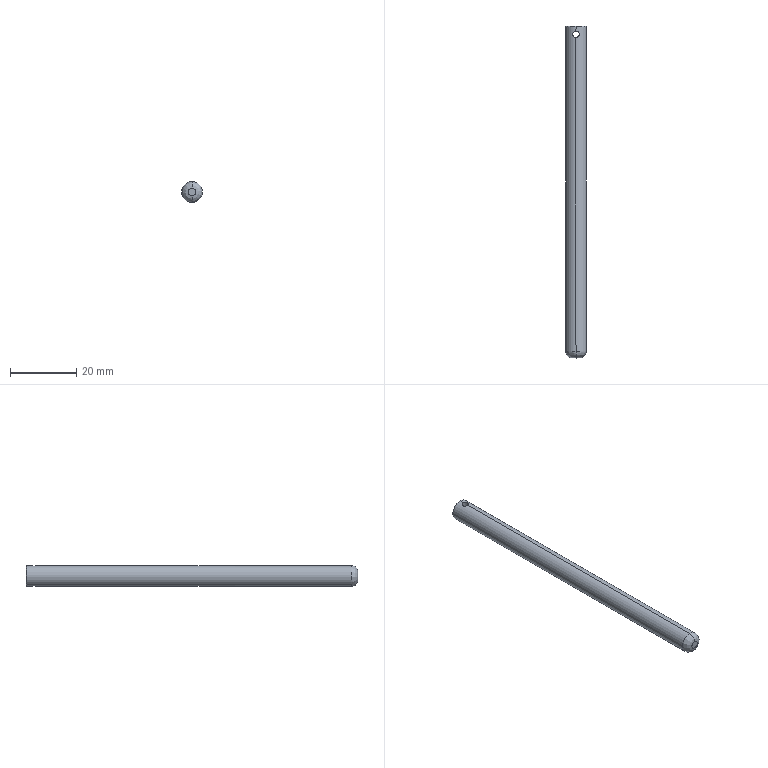Part | STEP file | 1 solid | 10 faces | box 6.3 x 100 x 6.3 mm | volume 3083 mm3 | cylinder 4 | other 2 | cone 2 | plane 2 | commonest cylinder face diameters 2 x2 6.3 x2
STEP:
#1=CARTESIAN_POINT('',(0.,0.,0.));
#2=DIRECTION('',(0.,0.,1.));
#3=DIRECTION('',(1.,0.,0.));
#4=AXIS2_PLACEMENT_3D('',#1,#2,#3);
#5=CARTESIAN_POINT('',(0.,0.,-1.15));
#6=VERTEX_POINT('',#5);
#7=CARTESIAN_POINT('',(0.,0.,1.15));
#8=VERTEX_POINT('',#7);
#9=CARTESIAN_POINT('',(0.,0.,0.));
#10=DIRECTION('',(0.,-1.,0.));
#11=DIRECTION('',(0.,0.,1.));
#12=AXIS2_PLACEMENT_3D('',#9,#10,#11);
#13=CIRCLE('',#12,1.15);
#14=CARTESIAN_POINT('',(0.,0.,1.15));
#15=CARTESIAN_POINT('',(0.,0.,1.412));
#16=CARTESIAN_POINT('',(0.,0.04112,1.674));
#17=CARTESIAN_POINT('',(0.,0.1234,1.927));
#18=CARTESIAN_POINT('',(0.,0.2446,2.165));
#19=CARTESIAN_POINT('',(0.,0.4007,2.379));
#20=CARTESIAN_POINT('',(0.,0.7709,2.749));
#21=CARTESIAN_POINT('',(0.,0.9851,2.905));
#22=CARTESIAN_POINT('',(0.,1.223,3.027));
#23=CARTESIAN_POINT('',(0.,1.476,3.109));
#24=CARTESIAN_POINT('',(0.,1.738,3.15));
#25=CARTESIAN_POINT('',(0.,2.,3.15));
#26=B_SPLINE_CURVE_WITH_KNOTS('',6,(#14,#15,#16,#17,#18,#19,#20,#21,#22,#23,#24,#25),.UNSPECIFIED.,.F.,.F.,(7,5,7),(4.712,5.498,6.283),.UNSPECIFIED.);
#27=CARTESIAN_POINT('',(0.,2.,0.));
#28=DIRECTION('',(0.,1.,0.));
#29=AXIS1_PLACEMENT('',#27,#28);
#30=SURFACE_OF_REVOLUTION('',#26,#29);
#31=CARTESIAN_POINT('',(6.283,4.712));
#32=DIRECTION('',(-1.,0.));
#33=VECTOR('',#32,1.);
#34=LINE('',#31,#33);
#35=(GEOMETRIC_REPRESENTATION_CONTEXT(2)PARAMETRIC_REPRESENTATION_CONTEXT()REPRESENTATION_CONTEXT('',''));
#36=DEFINITIONAL_REPRESENTATION('',(#34),#35);
#37=PCURVE('',#30,#36);
#38=CARTESIAN_POINT('',(0.,0.,0.));
#39=DIRECTION('',(0.,1.,0.));
#40=DIRECTION('',(0.,0.,1.));
#41=AXIS2_PLACEMENT_3D('',#38,#39,#40);
#42=PLANE('',#41);
#43=CARTESIAN_POINT('',(1.15,0.));
#44=CARTESIAN_POINT('',(1.15,-1.992));
#45=CARTESIAN_POINT('',(-0.575,-0.9959));
#46=CARTESIAN_POINT('',(-2.3,0.));
#47=CARTESIAN_POINT('',(-0.575,0.9959));
#48=CARTESIAN_POINT('',(1.15,1.992));
#49=CARTESIAN_POINT('',(1.15,0.));
#50=(BOUNDED_CURVE()B_SPLINE_CURVE(2,(#43,#44,#45,#46,#47,#48,#49),.UNSPECIFIED.,.T.,.F.)B_SPLINE_CURVE_WITH_KNOTS((1,2,2,2,2,1),(-2.094,0.,2.094,4.189,6.283,8.378),.UNSPECIFIED.)CURVE()GEOMETRIC_REPRESENTATION_ITEM()RATIONAL_B_SPLINE_CURVE((1.,0.5,1.,0.5,1.,0.5,1.))REPRESENTATION_ITEM(''));
#51=(GEOMETRIC_REPRESENTATION_CONTEXT(2)PARAMETRIC_REPRESENTATION_CONTEXT()REPRESENTATION_CONTEXT('',''));
#52=DEFINITIONAL_REPRESENTATION('',(#50),#51);
#53=PCURVE('',#42,#52);
#54=SURFACE_CURVE('',#13,(#37,#53),.PCURVE_S1.);
#55=EDGE_CURVE('',#6,#8,#54,.T.);
#56=ORIENTED_EDGE('',*,*,#55,.F.);
#57=CARTESIAN_POINT('',(0.,2.,-3.15));
#58=VERTEX_POINT('',#57);
#59=CARTESIAN_POINT('',(0.,2.,-1.15));
#60=DIRECTION('',(1.,0.,0.));
#61=DIRECTION('',(0.,0.,-1.));
#62=AXIS2_PLACEMENT_3D('',#59,#60,#61);
#63=CIRCLE('',#62,2.);
#64=CARTESIAN_POINT('',(3.142,0.));
#65=DIRECTION('',(0.,1.));
#66=VECTOR('',#65,1.);
#67=LINE('',#64,#66);
#68=(GEOMETRIC_REPRESENTATION_CONTEXT(2)PARAMETRIC_REPRESENTATION_CONTEXT()REPRESENTATION_CONTEXT('',''));
#69=DEFINITIONAL_REPRESENTATION('',(#67),#68);
#70=PCURVE('',#30,#69);
#71=CARTESIAN_POINT('',(0.,0.,1.15));
#72=CARTESIAN_POINT('',(0.,0.,1.412));
#73=CARTESIAN_POINT('',(0.,0.04112,1.674));
#74=CARTESIAN_POINT('',(0.,0.1234,1.927));
#75=CARTESIAN_POINT('',(0.,0.2446,2.165));
#76=CARTESIAN_POINT('',(0.,0.4007,2.379));
#77=CARTESIAN_POINT('',(0.,0.7709,2.749));
#78=CARTESIAN_POINT('',(0.,0.9851,2.905));
#79=CARTESIAN_POINT('',(0.,1.223,3.027));
#80=CARTESIAN_POINT('',(0.,1.476,3.109));
#81=CARTESIAN_POINT('',(0.,1.738,3.15));
#82=CARTESIAN_POINT('',(0.,2.,3.15));
#83=B_SPLINE_CURVE_WITH_KNOTS('',6,(#71,#72,#73,#74,#75,#76,#77,#78,#79,#80,#81,#82),.UNSPECIFIED.,.F.,.F.,(7,5,7),(4.712,5.498,6.283),.UNSPECIFIED.);
#84=CARTESIAN_POINT('',(0.,2.,0.));
#85=DIRECTION('',(0.,1.,0.));
#86=AXIS1_PLACEMENT('',#84,#85);
#87=SURFACE_OF_REVOLUTION('',#83,#86);
#88=CARTESIAN_POINT('',(3.142,0.));
#89=DIRECTION('',(0.,1.));
#90=VECTOR('',#89,1.);
#91=LINE('',#88,#90);
#92=(GEOMETRIC_REPRESENTATION_CONTEXT(2)PARAMETRIC_REPRESENTATION_CONTEXT()REPRESENTATION_CONTEXT('',''));
#93=DEFINITIONAL_REPRESENTATION('',(#91),#92);
#94=PCURVE('',#87,#93);
#95=SURFACE_CURVE('',#63,(#70,#94),.PCURVE_S1.);
#96=EDGE_CURVE('',#6,#58,#95,.T.);
#97=ORIENTED_EDGE('',*,*,#96,.T.);
#98=CARTESIAN_POINT('',(0.,2.,3.15));
#99=VERTEX_POINT('',#98);
#100=CARTESIAN_POINT('',(0.,2.,0.));
#101=DIRECTION('',(0.,1.,0.));
#102=DIRECTION('',(0.,0.,1.));
#103=AXIS2_PLACEMENT_3D('',#100,#101,#102);
#104=CIRCLE('',#103,3.15);
#105=CARTESIAN_POINT('',(0.,6.283));
#106=DIRECTION('',(1.,0.));
#107=VECTOR('',#106,1.);
#108=LINE('',#105,#107);
#109=(GEOMETRIC_REPRESENTATION_CONTEXT(2)PARAMETRIC_REPRESENTATION_CONTEXT()REPRESENTATION_CONTEXT('',''));
#110=DEFINITIONAL_REPRESENTATION('',(#108),#109);
#111=PCURVE('',#30,#110);
#112=CARTESIAN_POINT('',(0.,100.,0.));
#113=DIRECTION('',(0.,-1.,0.));
#114=DIRECTION('',(0.,0.,-1.));
#115=AXIS2_PLACEMENT_3D('',#112,#113,#114);
#116=CYLINDRICAL_SURFACE('',#115,3.15);
#117=CARTESIAN_POINT('',(3.142,98.));
#118=DIRECTION('',(-1.,0.));
#119=VECTOR('',#118,1.);
#120=LINE('',#117,#119);
#121=(GEOMETRIC_REPRESENTATION_CONTEXT(2)PARAMETRIC_REPRESENTATION_CONTEXT()REPRESENTATION_CONTEXT('',''));
#122=DEFINITIONAL_REPRESENTATION('',(#120),#121);
#123=PCURVE('',#116,#122);
#124=SURFACE_CURVE('',#104,(#111,#123),.PCURVE_S1.);
#125=EDGE_CURVE('',#99,#58,#124,.T.);
#126=ORIENTED_EDGE('',*,*,#125,.F.);
#127=CARTESIAN_POINT('',(0.,2.,1.15));
#128=DIRECTION('',(-1.,0.,0.));
#129=DIRECTION('',(0.,0.,1.));
#130=AXIS2_PLACEMENT_3D('',#127,#128,#129);
#131=CIRCLE('',#130,2.);
#132=CARTESIAN_POINT('',(0.,0.));
#133=DIRECTION('',(0.,1.));
#134=VECTOR('',#133,1.);
#135=LINE('',#132,#134);
#136=(GEOMETRIC_REPRESENTATION_CONTEXT(2)PARAMETRIC_REPRESENTATION_CONTEXT()REPRESENTATION_CONTEXT('',''));
#137=DEFINITIONAL_REPRESENTATION('',(#135),#136);
#138=PCURVE('',#30,#137);
#139=CARTESIAN_POINT('',(6.283,0.));
#140=DIRECTION('',(0.,1.));
#141=VECTOR('',#140,1.);
#142=LINE('',#139,#141);
#143=(GEOMETRIC_REPRESENTATION_CONTEXT(2)PARAMETRIC_REPRESENTATION_CONTEXT()REPRESENTATION_CONTEXT('',''));
#144=DEFINITIONAL_REPRESENTATION('',(#142),#143);
#145=PCURVE('',#87,#144);
#146=SURFACE_CURVE('',#131,(#138,#145),.PCURVE_S1.);
#147=EDGE_CURVE('',#8,#99,#146,.T.);
#148=ORIENTED_EDGE('',*,*,#147,.F.);
#149=EDGE_LOOP('',(#56,#97,#126,#148));
#150=FACE_BOUND('',#149,.T.);
#151=ADVANCED_FACE('',(#150),#30,.T.);
#152=CARTESIAN_POINT('',(0.,100.,2.95));
#153=VERTEX_POINT('',#152);
#154=CARTESIAN_POINT('',(0.,100.,-2.95));
#155=VERTEX_POINT('',#154);
#156=CARTESIAN_POINT('',(0.,100.,0.));
#157=DIRECTION('',(0.,1.,0.));
#158=DIRECTION('',(0.,0.,1.));
#159=AXIS2_PLACEMENT_3D('',#156,#157,#158);
#160=CIRCLE('',#159,2.95);
#161=CARTESIAN_POINT('',(0.,100.,0.));
#162=DIRECTION('',(0.,-1.,0.));
#163=DIRECTION('',(0.,0.,-1.));
#164=AXIS2_PLACEMENT_3D('',#161,#162,#163);
#165=CONICAL_SURFACE('',#164,2.95,0.7854);
#166=CARTESIAN_POINT('',(3.142,0.));
#167=DIRECTION('',(-1.,0.));
#168=VECTOR('',#167,1.);
#169=LINE('',#166,#168);
#170=(GEOMETRIC_REPRESENTATION_CONTEXT(2)PARAMETRIC_REPRESENTATION_CONTEXT()REPRESENTATION_CONTEXT('',''));
#171=DEFINITIONAL_REPRESENTATION('',(#169),#170);
#172=PCURVE('',#165,#171);
#173=CARTESIAN_POINT('',(0.,100.,0.));
#174=DIRECTION('',(0.,1.,0.));
#175=DIRECTION('',(0.,0.,1.));
#176=AXIS2_PLACEMENT_3D('',#173,#174,#175);
#177=PLANE('',#176);
#178=CARTESIAN_POINT('',(0.,0.));
#179=DIRECTION('',(1.,0.));
#180=AXIS2_PLACEMENT_2D('',#178,#179);
#181=CIRCLE('',#180,2.95);
#182=(GEOMETRIC_REPRESENTATION_CONTEXT(2)PARAMETRIC_REPRESENTATION_CONTEXT()REPRESENTATION_CONTEXT('',''));
#183=DEFINITIONAL_REPRESENTATION('',(#181),#182);
#184=PCURVE('',#177,#183);
#185=SURFACE_CURVE('',#160,(#172,#184),.PCURVE_S1.);
#186=EDGE_CURVE('',#153,#155,#185,.T.);
#187=ORIENTED_EDGE('',*,*,#186,.F.);
#188=CARTESIAN_POINT('',(0.,99.8,3.15));
#189=VERTEX_POINT('',#188);
#190=CARTESIAN_POINT('',(0.,100.,2.95));
#191=DIRECTION('',(0.,-0.7071,0.7071));
#192=VECTOR('',#191,1.);
#193=LINE('',#190,#192);
#194=CARTESIAN_POINT('',(3.142,0.));
#195=DIRECTION('',(0.,1.));
#196=VECTOR('',#195,1.);
#197=LINE('',#194,#196);
#198=(GEOMETRIC_REPRESENTATION_CONTEXT(2)PARAMETRIC_REPRESENTATION_CONTEXT()REPRESENTATION_CONTEXT('',''));
#199=DEFINITIONAL_REPRESENTATION('',(#197),#198);
#200=PCURVE('',#165,#199);
#201=CARTESIAN_POINT('',(0.,100.,0.));
#202=DIRECTION('',(0.,-1.,0.));
#203=DIRECTION('',(0.,0.,-1.));
#204=AXIS2_PLACEMENT_3D('',#201,#202,#203);
#205=CONICAL_SURFACE('',#204,2.95,0.7854);
#206=CARTESIAN_POINT('',(3.142,0.));
#207=DIRECTION('',(0.,1.));
#208=VECTOR('',#207,1.);
#209=LINE('',#206,#208);
#210=(GEOMETRIC_REPRESENTATION_CONTEXT(2)PARAMETRIC_REPRESENTATION_CONTEXT()REPRESENTATION_CONTEXT('',''));
#211=DEFINITIONAL_REPRESENTATION('',(#209),#210);
#212=PCURVE('',#205,#211);
#213=SURFACE_CURVE('',#193,(#200,#212),.PCURVE_S1.);
#214=EDGE_CURVE('',#153,#189,#213,.T.);
#215=ORIENTED_EDGE('',*,*,#214,.T.);
#216=CARTESIAN_POINT('',(0.,99.8,-3.15));
#217=VERTEX_POINT('',#216);
#218=CARTESIAN_POINT('',(0.,99.8,0.));
#219=DIRECTION('',(0.,-1.,0.));
#220=DIRECTION('',(0.,0.,1.));
#221=AXIS2_PLACEMENT_3D('',#218,#219,#220);
#222=CIRCLE('',#221,3.15);
#223=CARTESIAN_POINT('',(-3.142,0.2));
#224=DIRECTION('',(1.,0.));
#225=VECTOR('',#224,1.);
#226=LINE('',#223,#225);
#227=(GEOMETRIC_REPRESENTATION_CONTEXT(2)PARAMETRIC_REPRESENTATION_CONTEXT()REPRESENTATION_CONTEXT('',''));
#228=DEFINITIONAL_REPRESENTATION('',(#226),#227);
#229=PCURVE('',#165,#228);
#230=CARTESIAN_POINT('',(-3.142,0.2));
#231=DIRECTION('',(1.,0.));
#232=VECTOR('',#231,1.);
#233=LINE('',#230,#232);
#234=(GEOMETRIC_REPRESENTATION_CONTEXT(2)PARAMETRIC_REPRESENTATION_CONTEXT()REPRESENTATION_CONTEXT('',''));
#235=DEFINITIONAL_REPRESENTATION('',(#233),#234);
#236=PCURVE('',#116,#235);
#237=SURFACE_CURVE('',#222,(#229,#236),.PCURVE_S1.);
#238=EDGE_CURVE('',#217,#189,#237,.T.);
#239=ORIENTED_EDGE('',*,*,#238,.F.);
#240=CARTESIAN_POINT('',(0.,100.,-2.95));
#241=DIRECTION('',(0.,-0.7071,-0.7071));
#242=VECTOR('',#241,1.);
#243=LINE('',#240,#242);
#244=CARTESIAN_POINT('',(0.,0.));
#245=DIRECTION('',(0.,1.));
#246=VECTOR('',#245,1.);
#247=LINE('',#244,#246);
#248=(GEOMETRIC_REPRESENTATION_CONTEXT(2)PARAMETRIC_REPRESENTATION_CONTEXT()REPRESENTATION_CONTEXT('',''));
#249=DEFINITIONAL_REPRESENTATION('',(#247),#248);
#250=PCURVE('',#165,#249);
#251=CARTESIAN_POINT('',(6.283,0.));
#252=DIRECTION('',(0.,1.));
#253=VECTOR('',#252,1.);
#254=LINE('',#251,#253);
#255=(GEOMETRIC_REPRESENTATION_CONTEXT(2)PARAMETRIC_REPRESENTATION_CONTEXT()REPRESENTATION_CONTEXT('',''));
#256=DEFINITIONAL_REPRESENTATION('',(#254),#255);
#257=PCURVE('',#205,#256);
#258=SURFACE_CURVE('',#243,(#250,#257),.PCURVE_S1.);
#259=EDGE_CURVE('',#155,#217,#258,.T.);
#260=ORIENTED_EDGE('',*,*,#259,.F.);
#261=EDGE_LOOP('',(#187,#215,#239,#260));
#262=FACE_BOUND('',#261,.T.);
#263=ADVANCED_FACE('',(#262),#165,.T.);
#264=CARTESIAN_POINT('',(0.,96.5,-3.15));
#265=VERTEX_POINT('',#264);
#266=CARTESIAN_POINT('',(1.,97.5,-2.987));
#267=VERTEX_POINT('',#266);
#268=CARTESIAN_POINT('',(0.,96.5,-3.15));
#269=CARTESIAN_POINT('',(0.1311,96.5,-3.15));
#270=CARTESIAN_POINT('',(0.2634,96.527,-3.141));
#271=CARTESIAN_POINT('',(0.5046,96.627,-3.112));
#272=CARTESIAN_POINT('',(0.6148,96.701,-3.091));
#273=CARTESIAN_POINT('',(0.7994,96.885,-3.048));
#274=CARTESIAN_POINT('',(0.8727,96.994,-3.027));
#275=CARTESIAN_POINT('',(0.9739,97.238,-2.996));
#276=CARTESIAN_POINT('',(1.,97.368,-2.987));
#277=CARTESIAN_POINT('',(1.,97.5,-2.987));
#278=B_SPLINE_CURVE_WITH_KNOTS('',3,(#268,#269,#270,#271,#272,#273,#274,#275,#276,#277),.UNSPECIFIED.,.F.,.F.,(4,2,2,2,4),(0.003147,0.00354,0.003933,0.004327,0.00472),.UNSPECIFIED.);
#279=CARTESIAN_POINT('',(0.,97.5,-30.));
#280=DIRECTION('',(0.,0.,1.));
#281=DIRECTION('',(1.,0.,0.));
#282=AXIS2_PLACEMENT_3D('',#279,#280,#281);
#283=CYLINDRICAL_SURFACE('',#282,1.);
#284=CARTESIAN_POINT('',(4.712,26.85));
#285=CARTESIAN_POINT('',(4.736,26.85));
#286=CARTESIAN_POINT('',(4.784,26.851));
#287=CARTESIAN_POINT('',(4.856,26.853));
#288=CARTESIAN_POINT('',(4.928,26.857));
#289=CARTESIAN_POINT('',(4.999,26.863));
#290=CARTESIAN_POINT('',(5.071,26.869));
#291=CARTESIAN_POINT('',(5.142,26.877));
#292=CARTESIAN_POINT('',(5.213,26.887));
#293=CARTESIAN_POINT('',(5.284,26.897));
#294=CARTESIAN_POINT('',(5.356,26.908));
#295=CARTESIAN_POINT('',(5.427,26.919));
#296=CARTESIAN_POINT('',(5.498,26.93));
#297=CARTESIAN_POINT('',(5.569,26.942));
#298=CARTESIAN_POINT('',(5.64,26.953));
#299=CARTESIAN_POINT('',(5.711,26.964));
#300=CARTESIAN_POINT('',(5.782,26.975));
#301=CARTESIAN_POINT('',(5.853,26.984));
#302=CARTESIAN_POINT('',(5.925,26.993));
#303=CARTESIAN_POINT('',(5.997,27.));
#304=CARTESIAN_POINT('',(6.068,27.006));
#305=CARTESIAN_POINT('',(6.14,27.01));
#306=CARTESIAN_POINT('',(6.211,27.012));
#307=CARTESIAN_POINT('',(6.259,27.013));
#308=CARTESIAN_POINT('',(6.283,27.013));
#309=B_SPLINE_CURVE_WITH_KNOTS('',3,(#284,#285,#286,#287,#288,#289,#290,#291,#292,#293,#294,#295,#296,#297,#298,#299,#300,#301,#302,#303,#304,#305,#306,#307,#308),.UNSPECIFIED.,.F.,.F.,(4,1,1,1,1,1,1,1,1,1,1,1,1,1,1,1,1,1,1,1,1,1,4),(0.003147,0.003218,0.00329,0.003361,0.003433,0.003504,0.003576,0.003647,0.003719,0.00379,0.003862,0.003933,0.004005,0.004076,0.004148,0.004219,0.004291,0.004362,0.004434,0.004505,0.004577,0.004648,0.00472),.QUASI_UNIFORM_KNOTS.);
#310=(GEOMETRIC_REPRESENTATION_CONTEXT(2)PARAMETRIC_REPRESENTATION_CONTEXT()REPRESENTATION_CONTEXT('',''));
#311=DEFINITIONAL_REPRESENTATION('',(#309),#310);
#312=PCURVE('',#283,#311);
#313=CARTESIAN_POINT('',(0.,3.5));
#314=CARTESIAN_POINT('',(0.007565,3.5));
#315=CARTESIAN_POINT('',(0.02272,3.498));
#316=CARTESIAN_POINT('',(0.0454,3.49));
#317=CARTESIAN_POINT('',(0.06789,3.478));
#318=CARTESIAN_POINT('',(0.09004,3.46));
#319=CARTESIAN_POINT('',(0.1117,3.437));
#320=CARTESIAN_POINT('',(0.1328,3.41));
#321=CARTESIAN_POINT('',(0.1532,3.378));
#322=CARTESIAN_POINT('',(0.1728,3.341));
#323=CARTESIAN_POINT('',(0.1917,3.301));
#324=CARTESIAN_POINT('',(0.2096,3.256));
#325=CARTESIAN_POINT('',(0.2266,3.208));
#326=CARTESIAN_POINT('',(0.2424,3.156));
#327=CARTESIAN_POINT('',(0.257,3.1));
#328=CARTESIAN_POINT('',(0.2703,3.042));
#329=CARTESIAN_POINT('',(0.2823,2.981));
#330=CARTESIAN_POINT('',(0.293,2.917));
#331=CARTESIAN_POINT('',(0.3021,2.851));
#332=CARTESIAN_POINT('',(0.3097,2.783));
#333=CARTESIAN_POINT('',(0.3156,2.714));
#334=CARTESIAN_POINT('',(0.3199,2.643));
#335=CARTESIAN_POINT('',(0.3225,2.572));
#336=CARTESIAN_POINT('',(0.3231,2.524));
#337=CARTESIAN_POINT('',(0.3231,2.5));
#338=B_SPLINE_CURVE_WITH_KNOTS('',3,(#313,#314,#315,#316,#317,#318,#319,#320,#321,#322,#323,#324,#325,#326,#327,#328,#329,#330,#331,#332,#333,#334,#335,#336,#337),.UNSPECIFIED.,.F.,.F.,(4,1,1,1,1,1,1,1,1,1,1,1,1,1,1,1,1,1,1,1,1,1,4),(0.003147,0.003218,0.00329,0.003361,0.003433,0.003504,0.003576,0.003647,0.003719,0.00379,0.003862,0.003933,0.004005,0.004076,0.004148,0.004219,0.004291,0.004362,0.004434,0.004505,0.004577,0.004648,0.00472),.QUASI_UNIFORM_KNOTS.);
#339=(GEOMETRIC_REPRESENTATION_CONTEXT(2)PARAMETRIC_REPRESENTATION_CONTEXT()REPRESENTATION_CONTEXT('',''));
#340=DEFINITIONAL_REPRESENTATION('',(#338),#339);
#341=PCURVE('',#116,#340);
#342=SURFACE_CURVE('',#278,(#312,#341),.PCURVE_S1.);
#343=EDGE_CURVE('',#265,#267,#342,.T.);
#344=ORIENTED_EDGE('',*,*,#343,.T.);
#345=CARTESIAN_POINT('',(1.,97.5,2.987));
#346=VERTEX_POINT('',#345);
#347=CARTESIAN_POINT('',(1.,97.5,-30.));
#348=DIRECTION('',(0.,0.,1.));
#349=VECTOR('',#348,1.);
#350=LINE('',#347,#349);
#351=CARTESIAN_POINT('',(6.283,0.));
#352=DIRECTION('',(0.,1.));
#353=VECTOR('',#352,1.);
#354=LINE('',#351,#353);
#355=(GEOMETRIC_REPRESENTATION_CONTEXT(2)PARAMETRIC_REPRESENTATION_CONTEXT()REPRESENTATION_CONTEXT('',''));
#356=DEFINITIONAL_REPRESENTATION('',(#354),#355);
#357=PCURVE('',#283,#356);
#358=CARTESIAN_POINT('',(0.,97.5,-30.));
#359=DIRECTION('',(0.,0.,1.));
#360=DIRECTION('',(1.,0.,0.));
#361=AXIS2_PLACEMENT_3D('',#358,#359,#360);
#362=CYLINDRICAL_SURFACE('',#361,1.);
#363=CARTESIAN_POINT('',(0.,0.));
#364=DIRECTION('',(0.,1.));
#365=VECTOR('',#364,1.);
#366=LINE('',#363,#365);
#367=(GEOMETRIC_REPRESENTATION_CONTEXT(2)PARAMETRIC_REPRESENTATION_CONTEXT()REPRESENTATION_CONTEXT('',''));
#368=DEFINITIONAL_REPRESENTATION('',(#366),#367);
#369=PCURVE('',#362,#368);
#370=SURFACE_CURVE('',#350,(#357,#369),.PCURVE_S1.);
#371=EDGE_CURVE('',#267,#346,#370,.T.);
#372=ORIENTED_EDGE('',*,*,#371,.T.);
#373=CARTESIAN_POINT('',(0.,96.5,3.15));
#374=VERTEX_POINT('',#373);
#375=CARTESIAN_POINT('',(1.,97.5,2.987));
#376=CARTESIAN_POINT('',(1.,97.367,2.987));
#377=CARTESIAN_POINT('',(0.9735,97.236,2.996));
#378=CARTESIAN_POINT('',(0.8727,96.995,3.027));
#379=CARTESIAN_POINT('',(0.7985,96.884,3.049));
#380=CARTESIAN_POINT('',(0.6151,96.701,3.091));
#381=CARTESIAN_POINT('',(0.5042,96.627,3.112));
#382=CARTESIAN_POINT('',(0.2637,96.527,3.141));
#383=CARTESIAN_POINT('',(0.1315,96.5,3.15));
#384=CARTESIAN_POINT('',(0.,96.5,3.15));
#385=B_SPLINE_CURVE_WITH_KNOTS('',3,(#375,#376,#377,#378,#379,#380,#381,#382,#383,#384),.UNSPECIFIED.,.F.,.F.,(4,2,2,2,4),(0.,0.0003935,0.0007869,0.00118,0.001574),.UNSPECIFIED.);
#386=CARTESIAN_POINT('',(6.283,32.987));
#387=CARTESIAN_POINT('',(6.259,32.987));
#388=CARTESIAN_POINT('',(6.211,32.988));
#389=CARTESIAN_POINT('',(6.139,32.99));
#390=CARTESIAN_POINT('',(6.067,32.995));
#391=CARTESIAN_POINT('',(5.996,33.));
#392=CARTESIAN_POINT('',(5.924,33.007));
#393=CARTESIAN_POINT('',(5.853,33.016));
#394=CARTESIAN_POINT('',(5.781,33.025));
#395=CARTESIAN_POINT('',(5.71,33.036));
#396=CARTESIAN_POINT('',(5.639,33.047));
#397=CARTESIAN_POINT('',(5.568,33.058));
#398=CARTESIAN_POINT('',(5.497,33.07));
#399=CARTESIAN_POINT('',(5.427,33.081));
#400=CARTESIAN_POINT('',(5.356,33.092));
#401=CARTESIAN_POINT('',(5.284,33.103));
#402=CARTESIAN_POINT('',(5.213,33.113));
#403=CARTESIAN_POINT('',(5.142,33.123));
#404=CARTESIAN_POINT('',(5.071,33.131));
#405=CARTESIAN_POINT('',(5.,33.137));
#406=CARTESIAN_POINT('',(4.928,33.143));
#407=CARTESIAN_POINT('',(4.856,33.147));
#408=CARTESIAN_POINT('',(4.784,33.149));
#409=CARTESIAN_POINT('',(4.736,33.15));
#410=CARTESIAN_POINT('',(4.712,33.15));
#411=B_SPLINE_CURVE_WITH_KNOTS('',3,(#386,#387,#388,#389,#390,#391,#392,#393,#394,#395,#396,#397,#398,#399,#400,#401,#402,#403,#404,#405,#406,#407,#408,#409,#410),.UNSPECIFIED.,.F.,.F.,(4,1,1,1,1,1,1,1,1,1,1,1,1,1,1,1,1,1,1,1,1,1,4),(0.,0.00007154,0.0001431,0.0002146,0.0002862,0.0003577,0.0004292,0.0005008,0.0005723,0.0006439,0.0007154,0.0007869,0.0008585,0.00093,0.001002,0.001073,0.001145,0.001216,0.001288,0.001359,0.001431,0.001502,0.001574),.QUASI_UNIFORM_KNOTS.);
#412=(GEOMETRIC_REPRESENTATION_CONTEXT(2)PARAMETRIC_REPRESENTATION_CONTEXT()REPRESENTATION_CONTEXT('',''));
#413=DEFINITIONAL_REPRESENTATION('',(#411),#412);
#414=PCURVE('',#283,#413);
#415=CARTESIAN_POINT('',(2.819,2.5));
#416=CARTESIAN_POINT('',(2.819,2.524));
#417=CARTESIAN_POINT('',(2.819,2.572));
#418=CARTESIAN_POINT('',(2.822,2.644));
#419=CARTESIAN_POINT('',(2.826,2.715));
#420=CARTESIAN_POINT('',(2.832,2.784));
#421=CARTESIAN_POINT('',(2.84,2.852));
#422=CARTESIAN_POINT('',(2.849,2.918));
#423=CARTESIAN_POINT('',(2.859,2.981));
#424=CARTESIAN_POINT('',(2.871,3.043));
#425=CARTESIAN_POINT('',(2.885,3.101));
#426=CARTESIAN_POINT('',(2.899,3.156));
#427=CARTESIAN_POINT('',(2.915,3.208));
#428=CARTESIAN_POINT('',(2.932,3.256));
#429=CARTESIAN_POINT('',(2.95,3.301));
#430=CARTESIAN_POINT('',(2.969,3.341));
#431=CARTESIAN_POINT('',(2.988,3.378));
#432=CARTESIAN_POINT('',(3.009,3.41));
#433=CARTESIAN_POINT('',(3.03,3.437));
#434=CARTESIAN_POINT('',(3.051,3.46));
#435=CARTESIAN_POINT('',(3.074,3.478));
#436=CARTESIAN_POINT('',(3.096,3.49));
#437=CARTESIAN_POINT('',(3.119,3.498));
#438=CARTESIAN_POINT('',(3.134,3.5));
#439=CARTESIAN_POINT('',(3.142,3.5));
#440=B_SPLINE_CURVE_WITH_KNOTS('',3,(#415,#416,#417,#418,#419,#420,#421,#422,#423,#424,#425,#426,#427,#428,#429,#430,#431,#432,#433,#434,#435,#436,#437,#438,#439),.UNSPECIFIED.,.F.,.F.,(4,1,1,1,1,1,1,1,1,1,1,1,1,1,1,1,1,1,1,1,1,1,4),(0.,0.00007154,0.0001431,0.0002146,0.0002862,0.0003577,0.0004292,0.0005008,0.0005723,0.0006439,0.0007154,0.0007869,0.0008585,0.00093,0.001002,0.001073,0.001145,0.001216,0.001288,0.001359,0.001431,0.001502,0.001574),.QUASI_UNIFORM_KNOTS.);
#441=(GEOMETRIC_REPRESENTATION_CONTEXT(2)PARAMETRIC_REPRESENTATION_CONTEXT()REPRESENTATION_CONTEXT('',''));
#442=DEFINITIONAL_REPRESENTATION('',(#440),#441);
#443=PCURVE('',#116,#442);
#444=SURFACE_CURVE('',#385,(#414,#443),.PCURVE_S1.);
#445=EDGE_CURVE('',#346,#374,#444,.T.);
#446=ORIENTED_EDGE('',*,*,#445,.T.);
#447=CARTESIAN_POINT('',(-1.,97.5,2.987));
#448=VERTEX_POINT('',#447);
#449=CARTESIAN_POINT('',(0.,96.5,3.15));
#450=CARTESIAN_POINT('',(-0.1314,96.5,3.15));
#451=CARTESIAN_POINT('',(-0.2628,96.526,3.141));
#452=CARTESIAN_POINT('',(-0.506,96.627,3.112));
#453=CARTESIAN_POINT('',(-0.6156,96.701,3.091));
#454=CARTESIAN_POINT('',(-0.7998,96.886,3.048));
#455=CARTESIAN_POINT('',(-0.8734,96.996,3.027));
#456=CARTESIAN_POINT('',(-0.9735,97.237,2.996));
#457=CARTESIAN_POINT('',(-1.,97.369,2.987));
#458=CARTESIAN_POINT('',(-1.,97.5,2.987));
#459=B_SPLINE_CURVE_WITH_KNOTS('',3,(#449,#450,#451,#452,#453,#454,#455,#456,#457,#458),.UNSPECIFIED.,.F.,.F.,(4,2,2,2,4),(0.001574,0.001967,0.00236,0.002754,0.003147),.UNSPECIFIED.);
#460=CARTESIAN_POINT('',(4.712,33.15));
#461=CARTESIAN_POINT('',(4.688,33.15));
#462=CARTESIAN_POINT('',(4.641,33.149));
#463=CARTESIAN_POINT('',(4.569,33.147));
#464=CARTESIAN_POINT('',(4.497,33.143));
#465=CARTESIAN_POINT('',(4.426,33.137));
#466=CARTESIAN_POINT('',(4.354,33.131));
#467=CARTESIAN_POINT('',(4.282,33.122));
#468=CARTESIAN_POINT('',(4.21,33.113));
#469=CARTESIAN_POINT('',(4.139,33.103));
#470=CARTESIAN_POINT('',(4.068,33.092));
#471=CARTESIAN_POINT('',(3.997,33.081));
#472=CARTESIAN_POINT('',(3.926,33.069));
#473=CARTESIAN_POINT('',(3.855,33.058));
#474=CARTESIAN_POINT('',(3.784,33.047));
#475=CARTESIAN_POINT('',(3.713,33.036));
#476=CARTESIAN_POINT('',(3.642,33.025));
#477=CARTESIAN_POINT('',(3.571,33.016));
#478=CARTESIAN_POINT('',(3.5,33.007));
#479=CARTESIAN_POINT('',(3.428,33.));
#480=CARTESIAN_POINT('',(3.357,32.995));
#481=CARTESIAN_POINT('',(3.285,32.99));
#482=CARTESIAN_POINT('',(3.213,32.988));
#483=CARTESIAN_POINT('',(3.165,32.987));
#484=CARTESIAN_POINT('',(3.142,32.987));
#485=B_SPLINE_CURVE_WITH_KNOTS('',3,(#460,#461,#462,#463,#464,#465,#466,#467,#468,#469,#470,#471,#472,#473,#474,#475,#476,#477,#478,#479,#480,#481,#482,#483,#484),.UNSPECIFIED.,.F.,.F.,(4,1,1,1,1,1,1,1,1,1,1,1,1,1,1,1,1,1,1,1,1,1,4),(0.001574,0.001645,0.001717,0.001788,0.00186,0.001931,0.002003,0.002074,0.002146,0.002217,0.002289,0.00236,0.002432,0.002503,0.002575,0.002646,0.002718,0.002789,0.002861,0.002932,0.003004,0.003075,0.003147),.QUASI_UNIFORM_KNOTS.);
#486=(GEOMETRIC_REPRESENTATION_CONTEXT(2)PARAMETRIC_REPRESENTATION_CONTEXT()REPRESENTATION_CONTEXT('',''));
#487=DEFINITIONAL_REPRESENTATION('',(#485),#486);
#488=PCURVE('',#283,#487);
#489=CARTESIAN_POINT('',(0.,100.,0.));
#490=DIRECTION('',(0.,-1.,0.));
#491=DIRECTION('',(0.,0.,-1.));
#492=AXIS2_PLACEMENT_3D('',#489,#490,#491);
#493=CYLINDRICAL_SURFACE('',#492,3.15);
#494=CARTESIAN_POINT('',(3.142,3.5));
#495=CARTESIAN_POINT('',(3.149,3.5));
#496=CARTESIAN_POINT('',(3.164,3.498));
#497=CARTESIAN_POINT('',(3.187,3.491));
#498=CARTESIAN_POINT('',(3.209,3.478));
#499=CARTESIAN_POINT('',(3.232,3.46));
#500=CARTESIAN_POINT('',(3.253,3.437));
#501=CARTESIAN_POINT('',(3.275,3.41));
#502=CARTESIAN_POINT('',(3.295,3.377));
#503=CARTESIAN_POINT('',(3.315,3.341));
#504=CARTESIAN_POINT('',(3.334,3.3));
#505=CARTESIAN_POINT('',(3.351,3.256));
#506=CARTESIAN_POINT('',(3.368,3.207));
#507=CARTESIAN_POINT('',(3.384,3.155));
#508=CARTESIAN_POINT('',(3.399,3.1));
#509=CARTESIAN_POINT('',(3.412,3.041));
#510=CARTESIAN_POINT('',(3.424,2.98));
#511=CARTESIAN_POINT('',(3.435,2.917));
#512=CARTESIAN_POINT('',(3.444,2.851));
#513=CARTESIAN_POINT('',(3.451,2.783));
#514=CARTESIAN_POINT('',(3.457,2.714));
#515=CARTESIAN_POINT('',(3.461,2.643));
#516=CARTESIAN_POINT('',(3.464,2.572));
#517=CARTESIAN_POINT('',(3.465,2.524));
#518=CARTESIAN_POINT('',(3.465,2.5));
#519=B_SPLINE_CURVE_WITH_KNOTS('',3,(#494,#495,#496,#497,#498,#499,#500,#501,#502,#503,#504,#505,#506,#507,#508,#509,#510,#511,#512,#513,#514,#515,#516,#517,#518),.UNSPECIFIED.,.F.,.F.,(4,1,1,1,1,1,1,1,1,1,1,1,1,1,1,1,1,1,1,1,1,1,4),(0.001574,0.001645,0.001717,0.001788,0.00186,0.001931,0.002003,0.002074,0.002146,0.002217,0.002289,0.00236,0.002432,0.002503,0.002575,0.002646,0.002718,0.002789,0.002861,0.002932,0.003004,0.003075,0.003147),.QUASI_UNIFORM_KNOTS.);
#520=(GEOMETRIC_REPRESENTATION_CONTEXT(2)PARAMETRIC_REPRESENTATION_CONTEXT()REPRESENTATION_CONTEXT('',''));
#521=DEFINITIONAL_REPRESENTATION('',(#519),#520);
#522=PCURVE('',#493,#521);
#523=SURFACE_CURVE('',#459,(#488,#522),.PCURVE_S1.);
#524=EDGE_CURVE('',#374,#448,#523,.T.);
#525=ORIENTED_EDGE('',*,*,#524,.T.);
#526=CARTESIAN_POINT('',(-1.,97.5,-2.987));
#527=VERTEX_POINT('',#526);
#528=CARTESIAN_POINT('',(-1.,97.5,-30.));
#529=DIRECTION('',(0.,0.,1.));
#530=VECTOR('',#529,1.);
#531=LINE('',#528,#530);
#532=CARTESIAN_POINT('',(3.142,0.));
#533=DIRECTION('',(0.,1.));
#534=VECTOR('',#533,1.);
#535=LINE('',#532,#534);
#536=(GEOMETRIC_REPRESENTATION_CONTEXT(2)PARAMETRIC_REPRESENTATION_CONTEXT()REPRESENTATION_CONTEXT('',''));
#537=DEFINITIONAL_REPRESENTATION('',(#535),#536);
#538=PCURVE('',#283,#537);
#539=CARTESIAN_POINT('',(3.142,0.));
#540=DIRECTION('',(0.,1.));
#541=VECTOR('',#540,1.);
#542=LINE('',#539,#541);
#543=(GEOMETRIC_REPRESENTATION_CONTEXT(2)PARAMETRIC_REPRESENTATION_CONTEXT()REPRESENTATION_CONTEXT('',''));
#544=DEFINITIONAL_REPRESENTATION('',(#542),#543);
#545=PCURVE('',#362,#544);
#546=SURFACE_CURVE('',#531,(#538,#545),.PCURVE_S1.);
#547=EDGE_CURVE('',#527,#448,#546,.T.);
#548=ORIENTED_EDGE('',*,*,#547,.F.);
#549=CARTESIAN_POINT('',(-1.,97.5,-2.987));
#550=CARTESIAN_POINT('',(-1.,97.369,-2.987));
#551=CARTESIAN_POINT('',(-0.9738,97.237,-2.996));
#552=CARTESIAN_POINT('',(-0.8726,96.994,-3.027));
#553=CARTESIAN_POINT('',(-0.7989,96.885,-3.048));
#554=CARTESIAN_POINT('',(-0.6145,96.7,-3.091));
#555=CARTESIAN_POINT('',(-0.5042,96.627,-3.112));
#556=CARTESIAN_POINT('',(-0.2633,96.527,-3.141));
#557=CARTESIAN_POINT('',(-0.1311,96.5,-3.15));
#558=CARTESIAN_POINT('',(0.,96.5,-3.15));
#559=B_SPLINE_CURVE_WITH_KNOTS('',3,(#549,#550,#551,#552,#553,#554,#555,#556,#557,#558),.UNSPECIFIED.,.F.,.F.,(4,2,2,2,4),(0.001574,0.001967,0.00236,0.002754,0.003147),.UNSPECIFIED.);
#560=CARTESIAN_POINT('',(3.142,27.013));
#561=CARTESIAN_POINT('',(3.165,27.013));
#562=CARTESIAN_POINT('',(3.213,27.012));
#563=CARTESIAN_POINT('',(3.285,27.01));
#564=CARTESIAN_POINT('',(3.357,27.006));
#565=CARTESIAN_POINT('',(3.428,27.));
#566=CARTESIAN_POINT('',(3.5,26.993));
#567=CARTESIAN_POINT('',(3.572,26.984));
#568=CARTESIAN_POINT('',(3.643,26.975));
#569=CARTESIAN_POINT('',(3.715,26.964));
#570=CARTESIAN_POINT('',(3.786,26.953));
#571=CARTESIAN_POINT('',(3.857,26.942));
#572=CARTESIAN_POINT('',(3.928,26.93));
#573=CARTESIAN_POINT('',(3.999,26.919));
#574=CARTESIAN_POINT('',(4.07,26.907));
#575=CARTESIAN_POINT('',(4.141,26.897));
#576=CARTESIAN_POINT('',(4.212,26.887));
#577=CARTESIAN_POINT('',(4.283,26.877));
#578=CARTESIAN_POINT('',(4.354,26.869));
#579=CARTESIAN_POINT('',(4.426,26.863));
#580=CARTESIAN_POINT('',(4.497,26.857));
#581=CARTESIAN_POINT('',(4.569,26.853));
#582=CARTESIAN_POINT('',(4.641,26.851));
#583=CARTESIAN_POINT('',(4.689,26.85));
#584=CARTESIAN_POINT('',(4.712,26.85));
#585=B_SPLINE_CURVE_WITH_KNOTS('',3,(#560,#561,#562,#563,#564,#565,#566,#567,#568,#569,#570,#571,#572,#573,#574,#575,#576,#577,#578,#579,#580,#581,#582,#583,#584),.UNSPECIFIED.,.F.,.F.,(4,1,1,1,1,1,1,1,1,1,1,1,1,1,1,1,1,1,1,1,1,1,4),(0.001574,0.001645,0.001717,0.001788,0.00186,0.001931,0.002003,0.002074,0.002146,0.002217,0.002289,0.00236,0.002432,0.002503,0.002575,0.002646,0.002718,0.002789,0.002861,0.002932,0.003004,0.003075,0.003147),.QUASI_UNIFORM_KNOTS.);
#586=(GEOMETRIC_REPRESENTATION_CONTEXT(2)PARAMETRIC_REPRESENTATION_CONTEXT()REPRESENTATION_CONTEXT('',''));
#587=DEFINITIONAL_REPRESENTATION('',(#585),#586);
#588=PCURVE('',#283,#587);
#589=CARTESIAN_POINT('',(5.96,2.5));
#590=CARTESIAN_POINT('',(5.96,2.524));
#591=CARTESIAN_POINT('',(5.961,2.572));
#592=CARTESIAN_POINT('',(5.963,2.643));
#593=CARTESIAN_POINT('',(5.968,2.714));
#594=CARTESIAN_POINT('',(5.974,2.783));
#595=CARTESIAN_POINT('',(5.981,2.851));
#596=CARTESIAN_POINT('',(5.99,2.918));
#597=CARTESIAN_POINT('',(6.001,2.981));
#598=CARTESIAN_POINT('',(6.013,3.043));
#599=CARTESIAN_POINT('',(6.026,3.101));
#600=CARTESIAN_POINT('',(6.041,3.156));
#601=CARTESIAN_POINT('',(6.057,3.208));
#602=CARTESIAN_POINT('',(6.074,3.257));
#603=CARTESIAN_POINT('',(6.092,3.301));
#604=CARTESIAN_POINT('',(6.11,3.342));
#605=CARTESIAN_POINT('',(6.13,3.378));
#606=CARTESIAN_POINT('',(6.151,3.41));
#607=CARTESIAN_POINT('',(6.172,3.437));
#608=CARTESIAN_POINT('',(6.193,3.46));
#609=CARTESIAN_POINT('',(6.215,3.478));
#610=CARTESIAN_POINT('',(6.238,3.49));
#611=CARTESIAN_POINT('',(6.26,3.498));
#612=CARTESIAN_POINT('',(6.276,3.5));
#613=CARTESIAN_POINT('',(6.283,3.5));
#614=B_SPLINE_CURVE_WITH_KNOTS('',3,(#589,#590,#591,#592,#593,#594,#595,#596,#597,#598,#599,#600,#601,#602,#603,#604,#605,#606,#607,#608,#609,#610,#611,#612,#613),.UNSPECIFIED.,.F.,.F.,(4,1,1,1,1,1,1,1,1,1,1,1,1,1,1,1,1,1,1,1,1,1,4),(0.001574,0.001645,0.001717,0.001788,0.00186,0.001931,0.002003,0.002074,0.002146,0.002217,0.002289,0.00236,0.002432,0.002503,0.002575,0.002646,0.002718,0.002789,0.002861,0.002932,0.003004,0.003075,0.003147),.QUASI_UNIFORM_KNOTS.);
#615=(GEOMETRIC_REPRESENTATION_CONTEXT(2)PARAMETRIC_REPRESENTATION_CONTEXT()REPRESENTATION_CONTEXT('',''));
#616=DEFINITIONAL_REPRESENTATION('',(#614),#615);
#617=PCURVE('',#493,#616);
#618=SURFACE_CURVE('',#559,(#588,#617),.PCURVE_S1.);
#619=EDGE_CURVE('',#527,#265,#618,.T.);
#620=ORIENTED_EDGE('',*,*,#619,.T.);
#621=EDGE_LOOP('',(#344,#372,#446,#525,#548,#620));
#622=FACE_BOUND('',#621,.F.);
#623=ADVANCED_FACE('',(#622),#283,.F.);
#624=ORIENTED_EDGE('',*,*,#238,.T.);
#625=CARTESIAN_POINT('',(0.,98.5,3.15));
#626=VERTEX_POINT('',#625);
#627=CARTESIAN_POINT('',(0.,100.,3.15));
#628=DIRECTION('',(0.,-1.,0.));
#629=VECTOR('',#628,1.);
#630=LINE('',#627,#629);
#631=CARTESIAN_POINT('',(3.142,0.));
#632=DIRECTION('',(0.,1.));
#633=VECTOR('',#632,1.);
#634=LINE('',#631,#633);
#635=(GEOMETRIC_REPRESENTATION_CONTEXT(2)PARAMETRIC_REPRESENTATION_CONTEXT()REPRESENTATION_CONTEXT('',''));
#636=DEFINITIONAL_REPRESENTATION('',(#634),#635);
#637=PCURVE('',#116,#636);
#638=CARTESIAN_POINT('',(3.142,0.));
#639=DIRECTION('',(0.,1.));
#640=VECTOR('',#639,1.);
#641=LINE('',#638,#640);
#642=(GEOMETRIC_REPRESENTATION_CONTEXT(2)PARAMETRIC_REPRESENTATION_CONTEXT()REPRESENTATION_CONTEXT('',''));
#643=DEFINITIONAL_REPRESENTATION('',(#641),#642);
#644=PCURVE('',#493,#643);
#645=SURFACE_CURVE('',#630,(#637,#644),.PCURVE_S1.);
#646=EDGE_CURVE('',#189,#626,#645,.T.);
#647=ORIENTED_EDGE('',*,*,#646,.T.);
#648=CARTESIAN_POINT('',(0.,98.5,3.15));
#649=CARTESIAN_POINT('',(0.1318,98.5,3.15));
#650=CARTESIAN_POINT('',(0.2637,98.473,3.141));
#651=CARTESIAN_POINT('',(0.5046,98.373,3.112));
#652=CARTESIAN_POINT('',(0.6154,98.299,3.091));
#653=CARTESIAN_POINT('',(0.7987,98.116,3.049));
#654=CARTESIAN_POINT('',(0.8728,98.005,3.027));
#655=CARTESIAN_POINT('',(0.9734,97.764,2.996));
#656=CARTESIAN_POINT('',(1.,97.633,2.987));
#657=CARTESIAN_POINT('',(1.,97.5,2.987));
#658=B_SPLINE_CURVE_WITH_KNOTS('',3,(#648,#649,#650,#651,#652,#653,#654,#655,#656,#657),.UNSPECIFIED.,.F.,.F.,(4,2,2,2,4),(0.00472,0.005113,0.005506,0.0059,0.006293),.UNSPECIFIED.);
#659=CARTESIAN_POINT('',(3.142,1.5));
#660=CARTESIAN_POINT('',(3.134,1.5));
#661=CARTESIAN_POINT('',(3.119,1.502));
#662=CARTESIAN_POINT('',(3.096,1.51));
#663=CARTESIAN_POINT('',(3.074,1.522));
#664=CARTESIAN_POINT('',(3.051,1.54));
#665=CARTESIAN_POINT('',(3.03,1.563));
#666=CARTESIAN_POINT('',(3.009,1.59));
#667=CARTESIAN_POINT('',(2.988,1.622));
#668=CARTESIAN_POINT('',(2.969,1.659));
#669=CARTESIAN_POINT('',(2.95,1.699));
#670=CARTESIAN_POINT('',(2.932,1.744));
#671=CARTESIAN_POINT('',(2.915,1.792));
#672=CARTESIAN_POINT('',(2.899,1.844));
#673=CARTESIAN_POINT('',(2.885,1.899));
#674=CARTESIAN_POINT('',(2.871,1.958));
#675=CARTESIAN_POINT('',(2.859,2.019));
#676=CARTESIAN_POINT('',(2.849,2.082));
#677=CARTESIAN_POINT('',(2.84,2.148));
#678=CARTESIAN_POINT('',(2.832,2.216));
#679=CARTESIAN_POINT('',(2.826,2.285));
#680=CARTESIAN_POINT('',(2.822,2.356));
#681=CARTESIAN_POINT('',(2.819,2.428));
#682=CARTESIAN_POINT('',(2.819,2.476));
#683=CARTESIAN_POINT('',(2.819,2.5));
#684=B_SPLINE_CURVE_WITH_KNOTS('',3,(#659,#660,#661,#662,#663,#664,#665,#666,#667,#668,#669,#670,#671,#672,#673,#674,#675,#676,#677,#678,#679,#680,#681,#682,#683),.UNSPECIFIED.,.F.,.F.,(4,1,1,1,1,1,1,1,1,1,1,1,1,1,1,1,1,1,1,1,1,1,4),(0.00472,0.004791,0.004863,0.004934,0.005006,0.005077,0.005149,0.00522,0.005292,0.005363,0.005435,0.005506,0.005578,0.005649,0.005721,0.005792,0.005864,0.005935,0.006007,0.006078,0.00615,0.006221,0.006293),.QUASI_UNIFORM_KNOTS.);
#685=(GEOMETRIC_REPRESENTATION_CONTEXT(2)PARAMETRIC_REPRESENTATION_CONTEXT()REPRESENTATION_CONTEXT('',''));
#686=DEFINITIONAL_REPRESENTATION('',(#684),#685);
#687=PCURVE('',#116,#686);
#688=CARTESIAN_POINT('',(1.571,33.15));
#689=CARTESIAN_POINT('',(1.547,33.15));
#690=CARTESIAN_POINT('',(1.499,33.149));
#691=CARTESIAN_POINT('',(1.427,33.147));
#692=CARTESIAN_POINT('',(1.355,33.143));
#693=CARTESIAN_POINT('',(1.284,33.137));
#694=CARTESIAN_POINT('',(1.212,33.131));
#695=CARTESIAN_POINT('',(1.141,33.122));
#696=CARTESIAN_POINT('',(1.07,33.113));
#697=CARTESIAN_POINT('',(0.9985,33.103));
#698=CARTESIAN_POINT('',(0.9273,33.092));
#699=CARTESIAN_POINT('',(0.8563,33.081));
#700=CARTESIAN_POINT('',(0.7855,33.07));
#701=CARTESIAN_POINT('',(0.7147,33.058));
#702=CARTESIAN_POINT('',(0.6438,33.047));
#703=CARTESIAN_POINT('',(0.5728,33.036));
#704=CARTESIAN_POINT('',(0.5016,33.025));
#705=CARTESIAN_POINT('',(0.4304,33.016));
#706=CARTESIAN_POINT('',(0.3591,33.007));
#707=CARTESIAN_POINT('',(0.2877,33.));
#708=CARTESIAN_POINT('',(0.2162,32.995));
#709=CARTESIAN_POINT('',(0.1444,32.99));
#710=CARTESIAN_POINT('',(0.07243,32.988));
#711=CARTESIAN_POINT('',(0.02419,32.987));
#712=CARTESIAN_POINT('',(0.,32.987));
#713=B_SPLINE_CURVE_WITH_KNOTS('',3,(#688,#689,#690,#691,#692,#693,#694,#695,#696,#697,#698,#699,#700,#701,#702,#703,#704,#705,#706,#707,#708,#709,#710,#711,#712),.UNSPECIFIED.,.F.,.F.,(4,1,1,1,1,1,1,1,1,1,1,1,1,1,1,1,1,1,1,1,1,1,4),(0.00472,0.004791,0.004863,0.004934,0.005006,0.005077,0.005149,0.00522,0.005292,0.005363,0.005435,0.005506,0.005578,0.005649,0.005721,0.005792,0.005864,0.005935,0.006007,0.006078,0.00615,0.006221,0.006293),.QUASI_UNIFORM_KNOTS.);
#714=(GEOMETRIC_REPRESENTATION_CONTEXT(2)PARAMETRIC_REPRESENTATION_CONTEXT()REPRESENTATION_CONTEXT('',''));
#715=DEFINITIONAL_REPRESENTATION('',(#713),#714);
#716=PCURVE('',#362,#715);
#717=SURFACE_CURVE('',#658,(#687,#716),.PCURVE_S1.);
#718=EDGE_CURVE('',#626,#346,#717,.T.);
#719=ORIENTED_EDGE('',*,*,#718,.T.);
#720=ORIENTED_EDGE('',*,*,#445,.T.);
#721=CARTESIAN_POINT('',(0.,100.,3.15));
#722=DIRECTION('',(0.,-1.,0.));
#723=VECTOR('',#722,1.);
#724=LINE('',#721,#723);
#725=CARTESIAN_POINT('',(3.142,0.));
#726=DIRECTION('',(0.,1.));
#727=VECTOR('',#726,1.);
#728=LINE('',#725,#727);
#729=(GEOMETRIC_REPRESENTATION_CONTEXT(2)PARAMETRIC_REPRESENTATION_CONTEXT()REPRESENTATION_CONTEXT('',''));
#730=DEFINITIONAL_REPRESENTATION('',(#728),#729);
#731=PCURVE('',#116,#730);
#732=CARTESIAN_POINT('',(3.142,0.));
#733=DIRECTION('',(0.,1.));
#734=VECTOR('',#733,1.);
#735=LINE('',#732,#734);
#736=(GEOMETRIC_REPRESENTATION_CONTEXT(2)PARAMETRIC_REPRESENTATION_CONTEXT()REPRESENTATION_CONTEXT('',''));
#737=DEFINITIONAL_REPRESENTATION('',(#735),#736);
#738=PCURVE('',#493,#737);
#739=SURFACE_CURVE('',#724,(#731,#738),.PCURVE_S1.);
#740=EDGE_CURVE('',#374,#99,#739,.T.);
#741=ORIENTED_EDGE('',*,*,#740,.T.);
#742=ORIENTED_EDGE('',*,*,#125,.T.);
#743=CARTESIAN_POINT('',(0.,100.,-3.15));
#744=DIRECTION('',(0.,-1.,0.));
#745=VECTOR('',#744,1.);
#746=LINE('',#743,#745);
#747=CARTESIAN_POINT('',(0.,0.));
#748=DIRECTION('',(0.,1.));
#749=VECTOR('',#748,1.);
#750=LINE('',#747,#749);
#751=(GEOMETRIC_REPRESENTATION_CONTEXT(2)PARAMETRIC_REPRESENTATION_CONTEXT()REPRESENTATION_CONTEXT('',''));
#752=DEFINITIONAL_REPRESENTATION('',(#750),#751);
#753=PCURVE('',#116,#752);
#754=CARTESIAN_POINT('',(6.283,0.));
#755=DIRECTION('',(0.,1.));
#756=VECTOR('',#755,1.);
#757=LINE('',#754,#756);
#758=(GEOMETRIC_REPRESENTATION_CONTEXT(2)PARAMETRIC_REPRESENTATION_CONTEXT()REPRESENTATION_CONTEXT('',''));
#759=DEFINITIONAL_REPRESENTATION('',(#757),#758);
#760=PCURVE('',#493,#759);
#761=SURFACE_CURVE('',#746,(#753,#760),.PCURVE_S1.);
#762=EDGE_CURVE('',#265,#58,#761,.T.);
#763=ORIENTED_EDGE('',*,*,#762,.F.);
#764=ORIENTED_EDGE('',*,*,#343,.T.);
#765=CARTESIAN_POINT('',(0.,98.5,-3.15));
#766=VERTEX_POINT('',#765);
#767=CARTESIAN_POINT('',(1.,97.5,-2.987));
#768=CARTESIAN_POINT('',(1.,97.632,-2.987));
#769=CARTESIAN_POINT('',(0.9734,97.764,-2.996));
#770=CARTESIAN_POINT('',(0.8732,98.004,-3.027));
#771=CARTESIAN_POINT('',(0.799,98.115,-3.048));
#772=CARTESIAN_POINT('',(0.6157,98.299,-3.091));
#773=CARTESIAN_POINT('',(0.5054,98.373,-3.112));
#774=CARTESIAN_POINT('',(0.2639,98.473,-3.141));
#775=CARTESIAN_POINT('',(0.133,98.5,-3.15));
#776=CARTESIAN_POINT('',(0.,98.5,-3.15));
#777=B_SPLINE_CURVE_WITH_KNOTS('',3,(#767,#768,#769,#770,#771,#772,#773,#774,#775,#776),.UNSPECIFIED.,.F.,.F.,(4,2,2,2,4),(0.00472,0.005113,0.005507,0.0059,0.006293),.UNSPECIFIED.);
#778=CARTESIAN_POINT('',(0.3231,2.5));
#779=CARTESIAN_POINT('',(0.3231,2.476));
#780=CARTESIAN_POINT('',(0.3225,2.428));
#781=CARTESIAN_POINT('',(0.3198,2.357));
#782=CARTESIAN_POINT('',(0.3155,2.286));
#783=CARTESIAN_POINT('',(0.3096,2.217));
#784=CARTESIAN_POINT('',(0.3021,2.149));
#785=CARTESIAN_POINT('',(0.293,2.083));
#786=CARTESIAN_POINT('',(0.2824,2.019));
#787=CARTESIAN_POINT('',(0.2704,1.958));
#788=CARTESIAN_POINT('',(0.257,1.9));
#789=CARTESIAN_POINT('',(0.2424,1.844));
#790=CARTESIAN_POINT('',(0.2267,1.793));
#791=CARTESIAN_POINT('',(0.2098,1.744));
#792=CARTESIAN_POINT('',(0.1919,1.7));
#793=CARTESIAN_POINT('',(0.1731,1.659));
#794=CARTESIAN_POINT('',(0.1534,1.623));
#795=CARTESIAN_POINT('',(0.133,1.59));
#796=CARTESIAN_POINT('',(0.1119,1.563));
#797=CARTESIAN_POINT('',(0.09029,1.54));
#798=CARTESIAN_POINT('',(0.06821,1.522));
#799=CARTESIAN_POINT('',(0.04575,1.51));
#800=CARTESIAN_POINT('',(0.02299,1.502));
#801=CARTESIAN_POINT('',(0.007679,1.5));
#802=CARTESIAN_POINT('',(0.,1.5));
#803=B_SPLINE_CURVE_WITH_KNOTS('',3,(#778,#779,#780,#781,#782,#783,#784,#785,#786,#787,#788,#789,#790,#791,#792,#793,#794,#795,#796,#797,#798,#799,#800,#801,#802),.UNSPECIFIED.,.F.,.F.,(4,1,1,1,1,1,1,1,1,1,1,1,1,1,1,1,1,1,1,1,1,1,4),(0.00472,0.004791,0.004863,0.004935,0.005006,0.005078,0.005149,0.005221,0.005292,0.005364,0.005435,0.005507,0.005578,0.00565,0.005721,0.005793,0.005864,0.005936,0.006007,0.006079,0.00615,0.006222,0.006293),.QUASI_UNIFORM_KNOTS.);
#804=(GEOMETRIC_REPRESENTATION_CONTEXT(2)PARAMETRIC_REPRESENTATION_CONTEXT()REPRESENTATION_CONTEXT('',''));
#805=DEFINITIONAL_REPRESENTATION('',(#803),#804);
#806=PCURVE('',#116,#805);
#807=CARTESIAN_POINT('',(0.,27.013));
#808=CARTESIAN_POINT('',(0.02396,27.013));
#809=CARTESIAN_POINT('',(0.0719,27.012));
#810=CARTESIAN_POINT('',(0.1438,27.01));
#811=CARTESIAN_POINT('',(0.2156,27.005));
#812=CARTESIAN_POINT('',(0.2872,27.));
#813=CARTESIAN_POINT('',(0.3586,26.993));
#814=CARTESIAN_POINT('',(0.4298,26.984));
#815=CARTESIAN_POINT('',(0.501,26.975));
#816=CARTESIAN_POINT('',(0.5722,26.964));
#817=CARTESIAN_POINT('',(0.6433,26.953));
#818=CARTESIAN_POINT('',(0.7143,26.942));
#819=CARTESIAN_POINT('',(0.7851,26.93));
#820=CARTESIAN_POINT('',(0.8558,26.919));
#821=CARTESIAN_POINT('',(0.9268,26.908));
#822=CARTESIAN_POINT('',(0.9978,26.897));
#823=CARTESIAN_POINT('',(1.069,26.887));
#824=CARTESIAN_POINT('',(1.14,26.878));
#825=CARTESIAN_POINT('',(1.212,26.869));
#826=CARTESIAN_POINT('',(1.283,26.863));
#827=CARTESIAN_POINT('',(1.355,26.857));
#828=CARTESIAN_POINT('',(1.426,26.853));
#829=CARTESIAN_POINT('',(1.498,26.851));
#830=CARTESIAN_POINT('',(1.547,26.85));
#831=CARTESIAN_POINT('',(1.571,26.85));
#832=B_SPLINE_CURVE_WITH_KNOTS('',3,(#807,#808,#809,#810,#811,#812,#813,#814,#815,#816,#817,#818,#819,#820,#821,#822,#823,#824,#825,#826,#827,#828,#829,#830,#831),.UNSPECIFIED.,.F.,.F.,(4,1,1,1,1,1,1,1,1,1,1,1,1,1,1,1,1,1,1,1,1,1,4),(0.00472,0.004791,0.004863,0.004935,0.005006,0.005078,0.005149,0.005221,0.005292,0.005364,0.005435,0.005507,0.005578,0.00565,0.005721,0.005793,0.005864,0.005936,0.006007,0.006079,0.00615,0.006222,0.006293),.QUASI_UNIFORM_KNOTS.);
#833=(GEOMETRIC_REPRESENTATION_CONTEXT(2)PARAMETRIC_REPRESENTATION_CONTEXT()REPRESENTATION_CONTEXT('',''));
#834=DEFINITIONAL_REPRESENTATION('',(#832),#833);
#835=PCURVE('',#362,#834);
#836=SURFACE_CURVE('',#777,(#806,#835),.PCURVE_S1.);
#837=EDGE_CURVE('',#267,#766,#836,.T.);
#838=ORIENTED_EDGE('',*,*,#837,.T.);
#839=CARTESIAN_POINT('',(0.,100.,-3.15));
#840=DIRECTION('',(0.,-1.,0.));
#841=VECTOR('',#840,1.);
#842=LINE('',#839,#841);
#843=CARTESIAN_POINT('',(0.,0.));
#844=DIRECTION('',(0.,1.));
#845=VECTOR('',#844,1.);
#846=LINE('',#843,#845);
#847=(GEOMETRIC_REPRESENTATION_CONTEXT(2)PARAMETRIC_REPRESENTATION_CONTEXT()REPRESENTATION_CONTEXT('',''));
#848=DEFINITIONAL_REPRESENTATION('',(#846),#847);
#849=PCURVE('',#116,#848);
#850=CARTESIAN_POINT('',(6.283,0.));
#851=DIRECTION('',(0.,1.));
#852=VECTOR('',#851,1.);
#853=LINE('',#850,#852);
#854=(GEOMETRIC_REPRESENTATION_CONTEXT(2)PARAMETRIC_REPRESENTATION_CONTEXT()REPRESENTATION_CONTEXT('',''));
#855=DEFINITIONAL_REPRESENTATION('',(#853),#854);
#856=PCURVE('',#493,#855);
#857=SURFACE_CURVE('',#842,(#849,#856),.PCURVE_S1.);
#858=EDGE_CURVE('',#217,#766,#857,.T.);
#859=ORIENTED_EDGE('',*,*,#858,.F.);
#860=EDGE_LOOP('',(#624,#647,#719,#720,#741,#742,#763,#764,#838,#859));
#861=FACE_BOUND('',#860,.T.);
#862=ADVANCED_FACE('',(#861),#116,.T.);
#863=ORIENTED_EDGE('',*,*,#646,.F.);
#864=CARTESIAN_POINT('',(0.,99.8,0.));
#865=DIRECTION('',(0.,-1.,0.));
#866=DIRECTION('',(0.,0.,1.));
#867=AXIS2_PLACEMENT_3D('',#864,#865,#866);
#868=CIRCLE('',#867,3.15);
#869=CARTESIAN_POINT('',(3.142,0.2));
#870=DIRECTION('',(1.,0.));
#871=VECTOR('',#870,1.);
#872=LINE('',#869,#871);
#873=(GEOMETRIC_REPRESENTATION_CONTEXT(2)PARAMETRIC_REPRESENTATION_CONTEXT()REPRESENTATION_CONTEXT('',''));
#874=DEFINITIONAL_REPRESENTATION('',(#872),#873);
#875=PCURVE('',#493,#874);
#876=CARTESIAN_POINT('',(3.142,0.2));
#877=DIRECTION('',(1.,0.));
#878=VECTOR('',#877,1.);
#879=LINE('',#876,#878);
#880=(GEOMETRIC_REPRESENTATION_CONTEXT(2)PARAMETRIC_REPRESENTATION_CONTEXT()REPRESENTATION_CONTEXT('',''));
#881=DEFINITIONAL_REPRESENTATION('',(#879),#880);
#882=PCURVE('',#205,#881);
#883=SURFACE_CURVE('',#868,(#875,#882),.PCURVE_S1.);
#884=EDGE_CURVE('',#189,#217,#883,.T.);
#885=ORIENTED_EDGE('',*,*,#884,.T.);
#886=ORIENTED_EDGE('',*,*,#858,.T.);
#887=CARTESIAN_POINT('',(0.,98.5,-3.15));
#888=CARTESIAN_POINT('',(-0.1331,98.5,-3.15));
#889=CARTESIAN_POINT('',(-0.2637,98.473,-3.141));
#890=CARTESIAN_POINT('',(-0.5056,98.373,-3.112));
#891=CARTESIAN_POINT('',(-0.616,98.298,-3.091));
#892=CARTESIAN_POINT('',(-0.7991,98.115,-3.048));
#893=CARTESIAN_POINT('',(-0.8734,98.004,-3.027));
#894=CARTESIAN_POINT('',(-0.9734,97.764,-2.996));
#895=CARTESIAN_POINT('',(-1.,97.631,-2.987));
#896=CARTESIAN_POINT('',(-1.,97.5,-2.987));
#897=B_SPLINE_CURVE_WITH_KNOTS('',3,(#887,#888,#889,#890,#891,#892,#893,#894,#895,#896),.UNSPECIFIED.,.F.,.F.,(4,2,2,2,4),(0.,0.0003935,0.000787,0.00118,0.001574),.UNSPECIFIED.);
#898=CARTESIAN_POINT('',(6.283,1.5));
#899=CARTESIAN_POINT('',(6.276,1.5));
#900=CARTESIAN_POINT('',(6.26,1.502));
#901=CARTESIAN_POINT('',(6.237,1.51));
#902=CARTESIAN_POINT('',(6.215,1.522));
#903=CARTESIAN_POINT('',(6.193,1.54));
#904=CARTESIAN_POINT('',(6.171,1.563));
#905=CARTESIAN_POINT('',(6.15,1.59));
#906=CARTESIAN_POINT('',(6.13,1.623));
#907=CARTESIAN_POINT('',(6.11,1.659));
#908=CARTESIAN_POINT('',(6.091,1.7));
#909=CARTESIAN_POINT('',(6.073,1.744));
#910=CARTESIAN_POINT('',(6.056,1.793));
#911=CARTESIAN_POINT('',(6.041,1.845));
#912=CARTESIAN_POINT('',(6.026,1.9));
#913=CARTESIAN_POINT('',(6.013,1.958));
#914=CARTESIAN_POINT('',(6.001,2.02));
#915=CARTESIAN_POINT('',(5.99,2.083));
#916=CARTESIAN_POINT('',(5.981,2.149));
#917=CARTESIAN_POINT('',(5.974,2.217));
#918=CARTESIAN_POINT('',(5.968,2.286));
#919=CARTESIAN_POINT('',(5.963,2.357));
#920=CARTESIAN_POINT('',(5.961,2.428));
#921=CARTESIAN_POINT('',(5.96,2.476));
#922=CARTESIAN_POINT('',(5.96,2.5));
#923=B_SPLINE_CURVE_WITH_KNOTS('',3,(#898,#899,#900,#901,#902,#903,#904,#905,#906,#907,#908,#909,#910,#911,#912,#913,#914,#915,#916,#917,#918,#919,#920,#921,#922),.UNSPECIFIED.,.F.,.F.,(4,1,1,1,1,1,1,1,1,1,1,1,1,1,1,1,1,1,1,1,1,1,4),(0.,0.00007154,0.0001431,0.0002146,0.0002862,0.0003577,0.0004293,0.0005008,0.0005723,0.0006439,0.0007154,0.000787,0.0008585,0.0009301,0.001002,0.001073,0.001145,0.001216,0.001288,0.001359,0.001431,0.001502,0.001574),.QUASI_UNIFORM_KNOTS.);
#924=(GEOMETRIC_REPRESENTATION_CONTEXT(2)PARAMETRIC_REPRESENTATION_CONTEXT()REPRESENTATION_CONTEXT('',''));
#925=DEFINITIONAL_REPRESENTATION('',(#923),#924);
#926=PCURVE('',#493,#925);
#927=CARTESIAN_POINT('',(1.571,26.85));
#928=CARTESIAN_POINT('',(1.595,26.85));
#929=CARTESIAN_POINT('',(1.643,26.851));
#930=CARTESIAN_POINT('',(1.715,26.853));
#931=CARTESIAN_POINT('',(1.787,26.857));
#932=CARTESIAN_POINT('',(1.858,26.863));
#933=CARTESIAN_POINT('',(1.93,26.869));
#934=CARTESIAN_POINT('',(2.001,26.878));
#935=CARTESIAN_POINT('',(2.073,26.887));
#936=CARTESIAN_POINT('',(2.144,26.897));
#937=CARTESIAN_POINT('',(2.215,26.908));
#938=CARTESIAN_POINT('',(2.286,26.919));
#939=CARTESIAN_POINT('',(2.357,26.93));
#940=CARTESIAN_POINT('',(2.428,26.942));
#941=CARTESIAN_POINT('',(2.499,26.953));
#942=CARTESIAN_POINT('',(2.57,26.964));
#943=CARTESIAN_POINT('',(2.641,26.975));
#944=CARTESIAN_POINT('',(2.712,26.984));
#945=CARTESIAN_POINT('',(2.783,26.993));
#946=CARTESIAN_POINT('',(2.854,27.));
#947=CARTESIAN_POINT('',(2.926,27.005));
#948=CARTESIAN_POINT('',(2.998,27.01));
#949=CARTESIAN_POINT('',(3.07,27.012));
#950=CARTESIAN_POINT('',(3.118,27.013));
#951=CARTESIAN_POINT('',(3.142,27.013));
#952=B_SPLINE_CURVE_WITH_KNOTS('',3,(#927,#928,#929,#930,#931,#932,#933,#934,#935,#936,#937,#938,#939,#940,#941,#942,#943,#944,#945,#946,#947,#948,#949,#950,#951),.UNSPECIFIED.,.F.,.F.,(4,1,1,1,1,1,1,1,1,1,1,1,1,1,1,1,1,1,1,1,1,1,4),(0.,0.00007154,0.0001431,0.0002146,0.0002862,0.0003577,0.0004293,0.0005008,0.0005723,0.0006439,0.0007154,0.000787,0.0008585,0.0009301,0.001002,0.001073,0.001145,0.001216,0.001288,0.001359,0.001431,0.001502,0.001574),.QUASI_UNIFORM_KNOTS.);
#953=(GEOMETRIC_REPRESENTATION_CONTEXT(2)PARAMETRIC_REPRESENTATION_CONTEXT()REPRESENTATION_CONTEXT('',''));
#954=DEFINITIONAL_REPRESENTATION('',(#952),#953);
#955=PCURVE('',#362,#954);
#956=SURFACE_CURVE('',#897,(#926,#955),.PCURVE_S1.);
#957=EDGE_CURVE('',#766,#527,#956,.T.);
#958=ORIENTED_EDGE('',*,*,#957,.T.);
#959=ORIENTED_EDGE('',*,*,#619,.T.);
#960=ORIENTED_EDGE('',*,*,#762,.T.);
#961=CARTESIAN_POINT('',(0.,2.,0.));
#962=DIRECTION('',(0.,1.,0.));
#963=DIRECTION('',(0.,0.,1.));
#964=AXIS2_PLACEMENT_3D('',#961,#962,#963);
#965=CIRCLE('',#964,3.15);
#966=CARTESIAN_POINT('',(9.425,98.));
#967=DIRECTION('',(-1.,0.));
#968=VECTOR('',#967,1.);
#969=LINE('',#966,#968);
#970=(GEOMETRIC_REPRESENTATION_CONTEXT(2)PARAMETRIC_REPRESENTATION_CONTEXT()REPRESENTATION_CONTEXT('',''));
#971=DEFINITIONAL_REPRESENTATION('',(#969),#970);
#972=PCURVE('',#493,#971);
#973=CARTESIAN_POINT('',(0.,6.283));
#974=DIRECTION('',(1.,0.));
#975=VECTOR('',#974,1.);
#976=LINE('',#973,#975);
#977=(GEOMETRIC_REPRESENTATION_CONTEXT(2)PARAMETRIC_REPRESENTATION_CONTEXT()REPRESENTATION_CONTEXT('',''));
#978=DEFINITIONAL_REPRESENTATION('',(#976),#977);
#979=PCURVE('',#87,#978);
#980=SURFACE_CURVE('',#965,(#972,#979),.PCURVE_S1.);
#981=EDGE_CURVE('',#58,#99,#980,.T.);
#982=ORIENTED_EDGE('',*,*,#981,.T.);
#983=ORIENTED_EDGE('',*,*,#740,.F.);
#984=ORIENTED_EDGE('',*,*,#524,.T.);
#985=CARTESIAN_POINT('',(-1.,97.5,2.987));
#986=CARTESIAN_POINT('',(-1.,97.631,2.987));
#987=CARTESIAN_POINT('',(-0.9735,97.763,2.996));
#988=CARTESIAN_POINT('',(-0.8732,98.004,3.027));
#989=CARTESIAN_POINT('',(-0.7995,98.115,3.048));
#990=CARTESIAN_POINT('',(-0.615,98.299,3.091));
#991=CARTESIAN_POINT('',(-0.5059,98.373,3.112));
#992=CARTESIAN_POINT('',(-0.2624,98.474,3.141));
#993=CARTESIAN_POINT('',(-0.1318,98.5,3.15));
#994=CARTESIAN_POINT('',(0.,98.5,3.15));
#995=B_SPLINE_CURVE_WITH_KNOTS('',3,(#985,#986,#987,#988,#989,#990,#991,#992,#993,#994),.UNSPECIFIED.,.F.,.F.,(4,2,2,2,4),(0.003147,0.00354,0.003933,0.004327,0.00472),.UNSPECIFIED.);
#996=CARTESIAN_POINT('',(3.465,2.5));
#997=CARTESIAN_POINT('',(3.465,2.476));
#998=CARTESIAN_POINT('',(3.464,2.428));
#999=CARTESIAN_POINT('',(3.461,2.357));
#1000=CARTESIAN_POINT('',(3.457,2.286));
#1001=CARTESIAN_POINT('',(3.451,2.217));
#1002=CARTESIAN_POINT('',(3.444,2.149));
#1003=CARTESIAN_POINT('',(3.435,2.083));
#1004=CARTESIAN_POINT('',(3.424,2.019));
#1005=CARTESIAN_POINT('',(3.412,1.958));
#1006=CARTESIAN_POINT('',(3.399,1.9));
#1007=CARTESIAN_POINT('',(3.384,1.845));
#1008=CARTESIAN_POINT('',(3.368,1.792));
#1009=CARTESIAN_POINT('',(3.351,1.744));
#1010=CARTESIAN_POINT('',(3.333,1.699));
#1011=CARTESIAN_POINT('',(3.315,1.659));
#1012=CARTESIAN_POINT('',(3.295,1.622));
#1013=CARTESIAN_POINT('',(3.275,1.59));
#1014=CARTESIAN_POINT('',(3.253,1.563));
#1015=CARTESIAN_POINT('',(3.232,1.54));
#1016=CARTESIAN_POINT('',(3.209,1.522));
#1017=CARTESIAN_POINT('',(3.187,1.509));
#1018=CARTESIAN_POINT('',(3.164,1.502));
#1019=CARTESIAN_POINT('',(3.149,1.5));
#1020=CARTESIAN_POINT('',(3.142,1.5));
#1021=B_SPLINE_CURVE_WITH_KNOTS('',3,(#996,#997,#998,#999,#1000,#1001,#1002,#1003,#1004,#1005,#1006,#1007,#1008,#1009,#1010,#1011,#1012,#1013,#1014,#1015,#1016,#1017,#1018,#1019,#1020),.UNSPECIFIED.,.F.,.F.,(4,1,1,1,1,1,1,1,1,1,1,1,1,1,1,1,1,1,1,1,1,1,4),(0.003147,0.003218,0.00329,0.003361,0.003433,0.003504,0.003576,0.003647,0.003719,0.00379,0.003862,0.003933,0.004005,0.004076,0.004148,0.004219,0.004291,0.004362,0.004434,0.004505,0.004577,0.004648,0.00472),.QUASI_UNIFORM_KNOTS.);
#1022=(GEOMETRIC_REPRESENTATION_CONTEXT(2)PARAMETRIC_REPRESENTATION_CONTEXT()REPRESENTATION_CONTEXT('',''));
#1023=DEFINITIONAL_REPRESENTATION('',(#1021),#1022);
#1024=PCURVE('',#493,#1023);
#1025=CARTESIAN_POINT('',(3.142,32.987));
#1026=CARTESIAN_POINT('',(3.118,32.987));
#1027=CARTESIAN_POINT('',(3.07,32.988));
#1028=CARTESIAN_POINT('',(2.998,32.99));
#1029=CARTESIAN_POINT('',(2.926,32.995));
#1030=CARTESIAN_POINT('',(2.855,33.));
#1031=CARTESIAN_POINT('',(2.783,33.007));
#1032=CARTESIAN_POINT('',(2.712,33.016));
#1033=CARTESIAN_POINT('',(2.641,33.025));
#1034=CARTESIAN_POINT('',(2.57,33.036));
#1035=CARTESIAN_POINT('',(2.499,33.047));
#1036=CARTESIAN_POINT('',(2.428,33.058));
#1037=CARTESIAN_POINT('',(2.356,33.07));
#1038=CARTESIAN_POINT('',(2.285,33.081));
#1039=CARTESIAN_POINT('',(2.214,33.092));
#1040=CARTESIAN_POINT('',(2.144,33.103));
#1041=CARTESIAN_POINT('',(2.072,33.113));
#1042=CARTESIAN_POINT('',(2.001,33.122));
#1043=CARTESIAN_POINT('',(1.929,33.131));
#1044=CARTESIAN_POINT('',(1.857,33.137));
#1045=CARTESIAN_POINT('',(1.786,33.143));
#1046=CARTESIAN_POINT('',(1.714,33.147));
#1047=CARTESIAN_POINT('',(1.643,33.149));
#1048=CARTESIAN_POINT('',(1.595,33.15));
#1049=CARTESIAN_POINT('',(1.571,33.15));
#1050=B_SPLINE_CURVE_WITH_KNOTS('',3,(#1025,#1026,#1027,#1028,#1029,#1030,#1031,#1032,#1033,#1034,#1035,#1036,#1037,#1038,#1039,#1040,#1041,#1042,#1043,#1044,#1045,#1046,#1047,#1048,#1049),.UNSPECIFIED.,.F.,.F.,(4,1,1,1,1,1,1,1,1,1,1,1,1,1,1,1,1,1,1,1,1,1,4),(0.003147,0.003218,0.00329,0.003361,0.003433,0.003504,0.003576,0.003647,0.003719,0.00379,0.003862,0.003933,0.004005,0.004076,0.004148,0.004219,0.004291,0.004362,0.004434,0.004505,0.004577,0.004648,0.00472),.QUASI_UNIFORM_KNOTS.);
#1051=(GEOMETRIC_REPRESENTATION_CONTEXT(2)PARAMETRIC_REPRESENTATION_CONTEXT()REPRESENTATION_CONTEXT('',''));
#1052=DEFINITIONAL_REPRESENTATION('',(#1050),#1051);
#1053=PCURVE('',#362,#1052);
#1054=SURFACE_CURVE('',#995,(#1024,#1053),.PCURVE_S1.);
#1055=EDGE_CURVE('',#448,#626,#1054,.T.);
#1056=ORIENTED_EDGE('',*,*,#1055,.T.);
#1057=EDGE_LOOP('',(#863,#885,#886,#958,#959,#960,#982,#983,#984,#1056));
#1058=FACE_BOUND('',#1057,.T.);
#1059=ADVANCED_FACE('',(#1058),#493,.T.);
#1060=CARTESIAN_POINT('',(0.,100.,0.));
#1061=DIRECTION('',(0.,1.,0.));
#1062=DIRECTION('',(0.,0.,1.));
#1063=AXIS2_PLACEMENT_3D('',#1060,#1061,#1062);
#1064=CIRCLE('',#1063,2.95);
#1065=CARTESIAN_POINT('',(0.,0.));
#1066=DIRECTION('',(1.,0.));
#1067=AXIS2_PLACEMENT_2D('',#1065,#1066);
#1068=CIRCLE('',#1067,2.95);
#1069=(GEOMETRIC_REPRESENTATION_CONTEXT(2)PARAMETRIC_REPRESENTATION_CONTEXT()REPRESENTATION_CONTEXT('',''));
#1070=DEFINITIONAL_REPRESENTATION('',(#1068),#1069);
#1071=PCURVE('',#177,#1070);
#1072=CARTESIAN_POINT('',(9.425,0.));
#1073=DIRECTION('',(-1.,0.));
#1074=VECTOR('',#1073,1.);
#1075=LINE('',#1072,#1074);
#1076=(GEOMETRIC_REPRESENTATION_CONTEXT(2)PARAMETRIC_REPRESENTATION_CONTEXT()REPRESENTATION_CONTEXT('',''));
#1077=DEFINITIONAL_REPRESENTATION('',(#1075),#1076);
#1078=PCURVE('',#205,#1077);
#1079=SURFACE_CURVE('',#1064,(#1071,#1078),.PCURVE_S1.);
#1080=EDGE_CURVE('',#155,#153,#1079,.T.);
#1081=ORIENTED_EDGE('',*,*,#1080,.T.);
#1082=ORIENTED_EDGE('',*,*,#186,.T.);
#1083=EDGE_LOOP('',(#1081,#1082));
#1084=FACE_BOUND('',#1083,.T.);
#1085=ADVANCED_FACE('',(#1084),#177,.T.);
#1086=CARTESIAN_POINT('',(0.,0.,0.));
#1087=DIRECTION('',(0.,-1.,0.));
#1088=DIRECTION('',(0.,0.,1.));
#1089=AXIS2_PLACEMENT_3D('',#1086,#1087,#1088);
#1090=CIRCLE('',#1089,1.15);
#1091=CARTESIAN_POINT('',(1.15,0.));
#1092=CARTESIAN_POINT('',(1.15,-1.992));
#1093=CARTESIAN_POINT('',(-0.575,-0.9959));
#1094=CARTESIAN_POINT('',(-2.3,0.));
#1095=CARTESIAN_POINT('',(-0.575,0.9959));
#1096=CARTESIAN_POINT('',(1.15,1.992));
#1097=CARTESIAN_POINT('',(1.15,0.));
#1098=(BOUNDED_CURVE()B_SPLINE_CURVE(2,(#1091,#1092,#1093,#1094,#1095,#1096,#1097),.UNSPECIFIED.,.T.,.F.)B_SPLINE_CURVE_WITH_KNOTS((1,2,2,2,2,1),(-2.094,0.,2.094,4.189,6.283,8.378),.UNSPECIFIED.)CURVE()GEOMETRIC_REPRESENTATION_ITEM()RATIONAL_B_SPLINE_CURVE((1.,0.5,1.,0.5,1.,0.5,1.))REPRESENTATION_ITEM(''));
#1099=(GEOMETRIC_REPRESENTATION_CONTEXT(2)PARAMETRIC_REPRESENTATION_CONTEXT()REPRESENTATION_CONTEXT('',''));
#1100=DEFINITIONAL_REPRESENTATION('',(#1098),#1099);
#1101=PCURVE('',#42,#1100);
#1102=CARTESIAN_POINT('',(6.283,4.712));
#1103=DIRECTION('',(-1.,0.));
#1104=VECTOR('',#1103,1.);
#1105=LINE('',#1102,#1104);
#1106=(GEOMETRIC_REPRESENTATION_CONTEXT(2)PARAMETRIC_REPRESENTATION_CONTEXT()REPRESENTATION_CONTEXT('',''));
#1107=DEFINITIONAL_REPRESENTATION('',(#1105),#1106);
#1108=PCURVE('',#87,#1107);
#1109=SURFACE_CURVE('',#1090,(#1101,#1108),.PCURVE_S1.);
#1110=EDGE_CURVE('',#8,#6,#1109,.T.);
#1111=ORIENTED_EDGE('',*,*,#1110,.T.);
#1112=ORIENTED_EDGE('',*,*,#55,.T.);
#1113=EDGE_LOOP('',(#1111,#1112));
#1114=FACE_BOUND('',#1113,.T.);
#1115=ADVANCED_FACE('',(#1114),#42,.F.);
#1116=ORIENTED_EDGE('',*,*,#1055,.T.);
#1117=ORIENTED_EDGE('',*,*,#718,.T.);
#1118=ORIENTED_EDGE('',*,*,#371,.F.);
#1119=ORIENTED_EDGE('',*,*,#837,.T.);
#1120=ORIENTED_EDGE('',*,*,#957,.T.);
#1121=ORIENTED_EDGE('',*,*,#547,.T.);
#1122=EDGE_LOOP('',(#1116,#1117,#1118,#1119,#1120,#1121));
#1123=FACE_BOUND('',#1122,.F.);
#1124=ADVANCED_FACE('',(#1123),#362,.F.);
#1125=ORIENTED_EDGE('',*,*,#214,.F.);
#1126=ORIENTED_EDGE('',*,*,#1080,.F.);
#1127=ORIENTED_EDGE('',*,*,#259,.T.);
#1128=ORIENTED_EDGE('',*,*,#884,.F.);
#1129=EDGE_LOOP('',(#1125,#1126,#1127,#1128));
#1130=FACE_BOUND('',#1129,.T.);
#1131=ADVANCED_FACE('',(#1130),#205,.T.);
#1132=ORIENTED_EDGE('',*,*,#96,.F.);
#1133=ORIENTED_EDGE('',*,*,#1110,.F.);
#1134=ORIENTED_EDGE('',*,*,#147,.T.);
#1135=ORIENTED_EDGE('',*,*,#981,.F.);
#1136=EDGE_LOOP('',(#1132,#1133,#1134,#1135));
#1137=FACE_BOUND('',#1136,.T.);
#1138=ADVANCED_FACE('',(#1137),#87,.T.);
#1139=CLOSED_SHELL('',(#151,#263,#623,#862,#1059,#1085,#1115,#1124,#1131,#1138));
#1140=MANIFOLD_SOLID_BREP('',#1139);
#1141=(LENGTH_UNIT()NAMED_UNIT(*)SI_UNIT(.MILLI.,.METRE.));
#1142=UNCERTAINTY_MEASURE_WITH_UNIT(LENGTH_MEASURE(0.00005),#1141,'','');
#1143=(NAMED_UNIT(*)PLANE_ANGLE_UNIT()SI_UNIT($,.RADIAN.));
#1144=(NAMED_UNIT(*)SI_UNIT($,.STERADIAN.)SOLID_ANGLE_UNIT());
#1145=(GEOMETRIC_REPRESENTATION_CONTEXT(3)GLOBAL_UNCERTAINTY_ASSIGNED_CONTEXT((#1142))GLOBAL_UNIT_ASSIGNED_CONTEXT((#1141,#1143,#1144))REPRESENTATION_CONTEXT('',''));
#1146=ADVANCED_BREP_SHAPE_REPRESENTATION('',(#4,#1140),#1145);